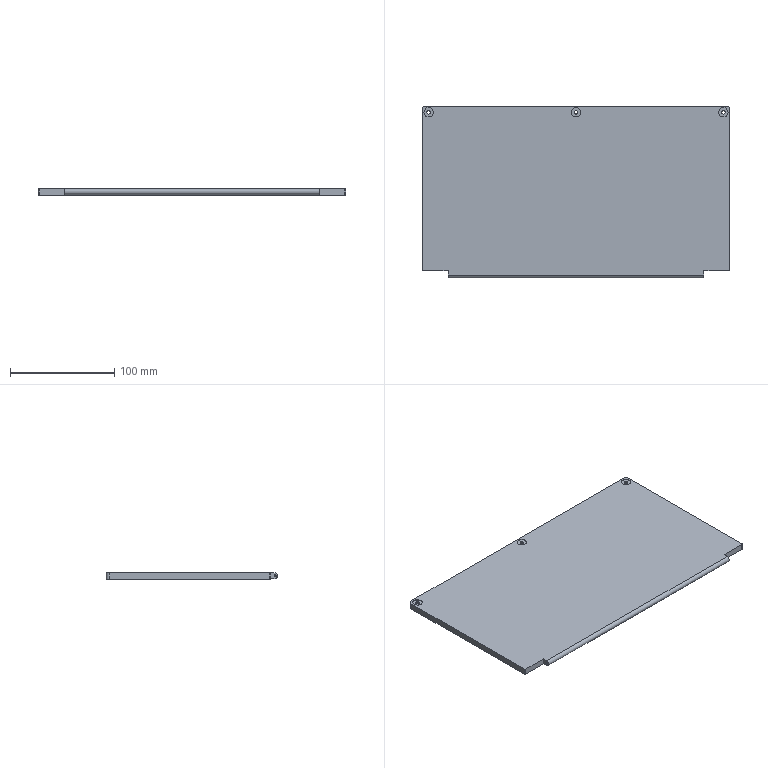Part | 1 solid | 65 faces | volume 116550 mm3 | cylinder 37 | plane 28 | commonest cylinder face diameters 6 x12 2 x6 3.3 x6 5 x6 9 x6 5.6 x1